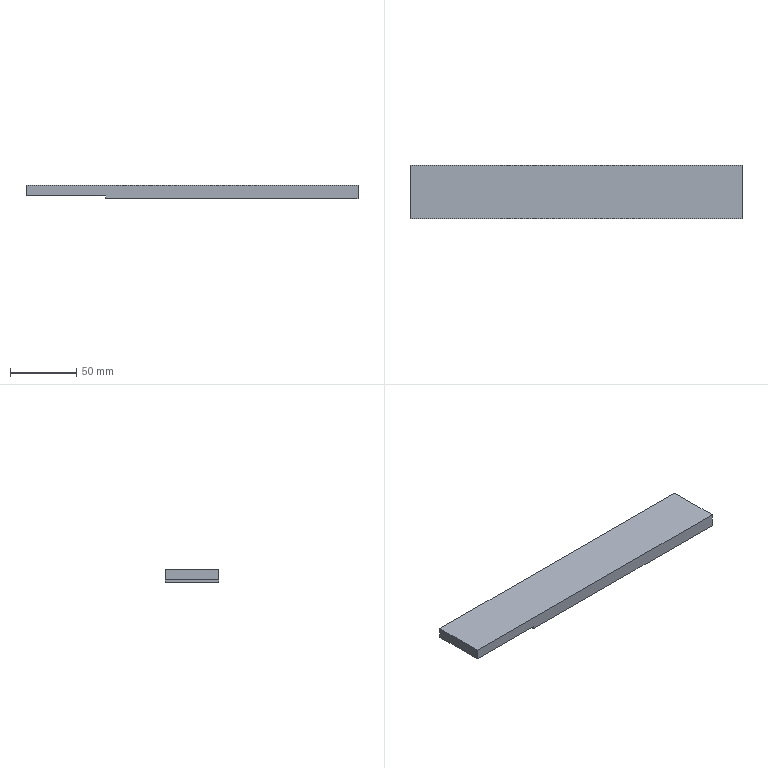Part | SolidWorks | features Extrusion 1, ICE 1 | 1 solid | 8 faces | box 250 x 40 x 10 mm | volume 95200 mm3 | plane 8
STEP:
#1=CARTESIAN_POINT('',(125.,-20.,-5.));
#2=VERTEX_POINT('',#1);
#3=CARTESIAN_POINT('',(125.,20.,-5.));
#4=VERTEX_POINT('',#3);
#5=CARTESIAN_POINT('',(125.,-20.,-5.));
#6=DIRECTION('',(0.,1.,0.));
#7=VECTOR('',#6,1000.);
#8=LINE('',#5,#7);
#9=EDGE_CURVE('',#2,#4,#8,.T.);
#10=ORIENTED_EDGE('',*,*,#9,.T.);
#11=CARTESIAN_POINT('',(125.,20.,5.));
#12=VERTEX_POINT('',#11);
#13=CARTESIAN_POINT('',(125.,20.,5.));
#14=DIRECTION('',(0.,0.,-1.));
#15=VECTOR('',#14,1000.);
#16=LINE('',#13,#15);
#17=EDGE_CURVE('',#12,#4,#16,.T.);
#18=ORIENTED_EDGE('',*,*,#17,.F.);
#19=CARTESIAN_POINT('',(125.,-20.,5.));
#20=VERTEX_POINT('',#19);
#21=CARTESIAN_POINT('',(125.,-20.,5.));
#22=DIRECTION('',(0.,1.,0.));
#23=VECTOR('',#22,1000.);
#24=LINE('',#21,#23);
#25=EDGE_CURVE('',#20,#12,#24,.T.);
#26=ORIENTED_EDGE('',*,*,#25,.F.);
#27=CARTESIAN_POINT('',(125.,-20.,5.));
#28=DIRECTION('',(0.,0.,-1.));
#29=VECTOR('',#28,1000.);
#30=LINE('',#27,#29);
#31=EDGE_CURVE('',#20,#2,#30,.T.);
#32=ORIENTED_EDGE('',*,*,#31,.T.);
#33=EDGE_LOOP('',(#10,#18,#26,#32));
#34=FACE_OUTER_BOUND('',#33,.T.);
#35=CARTESIAN_POINT('',(125.,-20.,5.));
#36=DIRECTION('',(-1.,0.,0.));
#37=DIRECTION('',(0.,0.,1.));
#38=AXIS2_PLACEMENT_3D('',#35,#36,#37);
#39=PLANE('',#38);
#40=ADVANCED_FACE('',(#34),#39,.F.);
#41=CARTESIAN_POINT('',(-65.,20.,-5.));
#42=VERTEX_POINT('',#41);
#43=CARTESIAN_POINT('',(-125.,20.,-5.));
#44=DIRECTION('',(-1.,0.,0.));
#45=VECTOR('',#44,1000.);
#46=LINE('',#43,#45);
#47=EDGE_CURVE('',#4,#42,#46,.T.);
#48=ORIENTED_EDGE('',*,*,#47,.T.);
#49=CARTESIAN_POINT('',(-65.,20.,-3.));
#50=VERTEX_POINT('',#49);
#51=CARTESIAN_POINT('',(-65.,20.,-3.));
#52=DIRECTION('',(0.,0.,-1.));
#53=VECTOR('',#52,1000.);
#54=LINE('',#51,#53);
#55=EDGE_CURVE('',#50,#42,#54,.T.);
#56=ORIENTED_EDGE('',*,*,#55,.F.);
#57=CARTESIAN_POINT('',(-125.,20.,-3.));
#58=VERTEX_POINT('',#57);
#59=CARTESIAN_POINT('',(-125.,20.,-3.));
#60=DIRECTION('',(1.,0.,0.));
#61=VECTOR('',#60,1000.);
#62=LINE('',#59,#61);
#63=EDGE_CURVE('',#58,#50,#62,.T.);
#64=ORIENTED_EDGE('',*,*,#63,.F.);
#65=CARTESIAN_POINT('',(-125.,20.,5.));
#66=VERTEX_POINT('',#65);
#67=CARTESIAN_POINT('',(-125.,20.,5.));
#68=DIRECTION('',(0.,0.,-1.));
#69=VECTOR('',#68,1000.);
#70=LINE('',#67,#69);
#71=EDGE_CURVE('',#66,#58,#70,.T.);
#72=ORIENTED_EDGE('',*,*,#71,.F.);
#73=CARTESIAN_POINT('',(-125.,20.,5.));
#74=DIRECTION('',(-1.,0.,0.));
#75=VECTOR('',#74,1000.);
#76=LINE('',#73,#75);
#77=EDGE_CURVE('',#12,#66,#76,.T.);
#78=ORIENTED_EDGE('',*,*,#77,.F.);
#79=ORIENTED_EDGE('',*,*,#17,.T.);
#80=EDGE_LOOP('',(#48,#56,#64,#72,#78,#79));
#81=FACE_OUTER_BOUND('',#80,.T.);
#82=CARTESIAN_POINT('',(-125.,20.,5.));
#83=DIRECTION('',(0.,-1.,0.));
#84=DIRECTION('',(0.,0.,-1.));
#85=AXIS2_PLACEMENT_3D('',#82,#83,#84);
#86=PLANE('',#85);
#87=ADVANCED_FACE('',(#81),#86,.F.);
#88=ORIENTED_EDGE('',*,*,#71,.T.);
#89=CARTESIAN_POINT('',(-125.,-20.,-3.));
#90=VERTEX_POINT('',#89);
#91=CARTESIAN_POINT('',(-125.,20.,-3.));
#92=DIRECTION('',(0.,1.,0.));
#93=VECTOR('',#92,1000.);
#94=LINE('',#91,#93);
#95=EDGE_CURVE('',#90,#58,#94,.T.);
#96=ORIENTED_EDGE('',*,*,#95,.F.);
#97=CARTESIAN_POINT('',(-125.,-20.,5.));
#98=VERTEX_POINT('',#97);
#99=CARTESIAN_POINT('',(-125.,-20.,5.));
#100=DIRECTION('',(0.,0.,-1.));
#101=VECTOR('',#100,1000.);
#102=LINE('',#99,#101);
#103=EDGE_CURVE('',#98,#90,#102,.T.);
#104=ORIENTED_EDGE('',*,*,#103,.F.);
#105=CARTESIAN_POINT('',(-125.,-20.,5.));
#106=DIRECTION('',(0.,-1.,0.));
#107=VECTOR('',#106,1000.);
#108=LINE('',#105,#107);
#109=EDGE_CURVE('',#66,#98,#108,.T.);
#110=ORIENTED_EDGE('',*,*,#109,.F.);
#111=EDGE_LOOP('',(#88,#96,#104,#110));
#112=FACE_OUTER_BOUND('',#111,.T.);
#113=CARTESIAN_POINT('',(-125.,-20.,5.));
#114=DIRECTION('',(1.,0.,0.));
#115=DIRECTION('',(0.,0.,-1.));
#116=AXIS2_PLACEMENT_3D('',#113,#114,#115);
#117=PLANE('',#116);
#118=ADVANCED_FACE('',(#112),#117,.F.);
#119=CARTESIAN_POINT('',(-65.,-20.,-3.));
#120=VERTEX_POINT('',#119);
#121=CARTESIAN_POINT('',(-125.,-20.,-3.));
#122=DIRECTION('',(-1.,0.,0.));
#123=VECTOR('',#122,1000.);
#124=LINE('',#121,#123);
#125=EDGE_CURVE('',#120,#90,#124,.T.);
#126=ORIENTED_EDGE('',*,*,#125,.F.);
#127=CARTESIAN_POINT('',(-65.,-20.,-5.));
#128=VERTEX_POINT('',#127);
#129=CARTESIAN_POINT('',(-65.,-20.,-3.));
#130=DIRECTION('',(0.,0.,-1.));
#131=VECTOR('',#130,1000.);
#132=LINE('',#129,#131);
#133=EDGE_CURVE('',#120,#128,#132,.T.);
#134=ORIENTED_EDGE('',*,*,#133,.T.);
#135=CARTESIAN_POINT('',(-125.,-20.,-5.));
#136=DIRECTION('',(1.,0.,0.));
#137=VECTOR('',#136,1000.);
#138=LINE('',#135,#137);
#139=EDGE_CURVE('',#128,#2,#138,.T.);
#140=ORIENTED_EDGE('',*,*,#139,.T.);
#141=ORIENTED_EDGE('',*,*,#31,.F.);
#142=CARTESIAN_POINT('',(-125.,-20.,5.));
#143=DIRECTION('',(1.,0.,0.));
#144=VECTOR('',#143,1000.);
#145=LINE('',#142,#144);
#146=EDGE_CURVE('',#98,#20,#145,.T.);
#147=ORIENTED_EDGE('',*,*,#146,.F.);
#148=ORIENTED_EDGE('',*,*,#103,.T.);
#149=EDGE_LOOP('',(#126,#134,#140,#141,#147,#148));
#150=FACE_OUTER_BOUND('',#149,.T.);
#151=CARTESIAN_POINT('',(-125.,-20.,5.));
#152=DIRECTION('',(0.,1.,0.));
#153=DIRECTION('',(0.,0.,1.));
#154=AXIS2_PLACEMENT_3D('',#151,#152,#153);
#155=PLANE('',#154);
#156=ADVANCED_FACE('',(#150),#155,.F.);
#157=ORIENTED_EDGE('',*,*,#25,.T.);
#158=ORIENTED_EDGE('',*,*,#77,.T.);
#159=ORIENTED_EDGE('',*,*,#109,.T.);
#160=ORIENTED_EDGE('',*,*,#146,.T.);
#161=EDGE_LOOP('',(#157,#158,#159,#160));
#162=FACE_OUTER_BOUND('',#161,.T.);
#163=CARTESIAN_POINT('',(0.,0.,5.));
#164=DIRECTION('',(0.,0.,-1.));
#165=DIRECTION('',(-1.,0.,0.));
#166=AXIS2_PLACEMENT_3D('',#163,#164,#165);
#167=PLANE('',#166);
#168=ADVANCED_FACE('',(#162),#167,.F.);
#169=CARTESIAN_POINT('',(-65.,20.,-5.));
#170=DIRECTION('',(0.,-1.,0.));
#171=VECTOR('',#170,1000.);
#172=LINE('',#169,#171);
#173=EDGE_CURVE('',#42,#128,#172,.T.);
#174=ORIENTED_EDGE('',*,*,#173,.F.);
#175=ORIENTED_EDGE('',*,*,#47,.F.);
#176=ORIENTED_EDGE('',*,*,#9,.F.);
#177=ORIENTED_EDGE('',*,*,#139,.F.);
#178=EDGE_LOOP('',(#174,#175,#176,#177));
#179=FACE_OUTER_BOUND('',#178,.T.);
#180=CARTESIAN_POINT('',(0.,0.,-5.));
#181=DIRECTION('',(0.,0.,-1.));
#182=DIRECTION('',(-1.,0.,0.));
#183=AXIS2_PLACEMENT_3D('',#180,#181,#182);
#184=PLANE('',#183);
#185=ADVANCED_FACE('',(#179),#184,.T.);
#186=ORIENTED_EDGE('',*,*,#173,.T.);
#187=ORIENTED_EDGE('',*,*,#133,.F.);
#188=CARTESIAN_POINT('',(-65.,20.,-3.));
#189=DIRECTION('',(0.,-1.,0.));
#190=VECTOR('',#189,1000.);
#191=LINE('',#188,#190);
#192=EDGE_CURVE('',#50,#120,#191,.T.);
#193=ORIENTED_EDGE('',*,*,#192,.F.);
#194=ORIENTED_EDGE('',*,*,#55,.T.);
#195=EDGE_LOOP('',(#186,#187,#193,#194));
#196=FACE_OUTER_BOUND('',#195,.T.);
#197=CARTESIAN_POINT('',(-65.,20.,-3.));
#198=DIRECTION('',(1.,0.,0.));
#199=DIRECTION('',(0.,0.,-1.));
#200=AXIS2_PLACEMENT_3D('',#197,#198,#199);
#201=PLANE('',#200);
#202=ADVANCED_FACE('',(#196),#201,.F.);
#203=ORIENTED_EDGE('',*,*,#95,.T.);
#204=ORIENTED_EDGE('',*,*,#63,.T.);
#205=ORIENTED_EDGE('',*,*,#192,.T.);
#206=ORIENTED_EDGE('',*,*,#125,.T.);
#207=EDGE_LOOP('',(#203,#204,#205,#206));
#208=FACE_OUTER_BOUND('',#207,.T.);
#209=CARTESIAN_POINT('',(0.,0.,-3.));
#210=DIRECTION('',(0.,0.,1.));
#211=DIRECTION('',(1.,0.,0.));
#212=AXIS2_PLACEMENT_3D('',#209,#210,#211);
#213=PLANE('',#212);
#214=ADVANCED_FACE('',(#208),#213,.F.);
#215=CLOSED_SHELL('',(#40,#87,#118,#156,#168,#185,#202,#214));
#216=MANIFOLD_SOLID_BREP('',#215);
#217=CARTESIAN_POINT('',(0.,0.,0.));
#218=DIRECTION('',(0.,0.,1.));
#219=DIRECTION('',(1.,0.,0.));
#220=AXIS2_PLACEMENT_3D('',#217,#218,#219);
#221=(LENGTH_UNIT()NAMED_UNIT(*)SI_UNIT(.MILLI.,.METRE.));
#222=UNCERTAINTY_MEASURE_WITH_UNIT(LENGTH_MEASURE(0.00001),#221,'','');
#223=(NAMED_UNIT(*)PLANE_ANGLE_UNIT()SI_UNIT($,.RADIAN.));
#224=(NAMED_UNIT(*)SI_UNIT($,.STERADIAN.)SOLID_ANGLE_UNIT());
#225=(GEOMETRIC_REPRESENTATION_CONTEXT(3)GLOBAL_UNCERTAINTY_ASSIGNED_CONTEXT((#222))GLOBAL_UNIT_ASSIGNED_CONTEXT((#221,#223,#224))REPRESENTATION_CONTEXT('',''));
#226=ADVANCED_BREP_SHAPE_REPRESENTATION('',(#216,#220),#225);